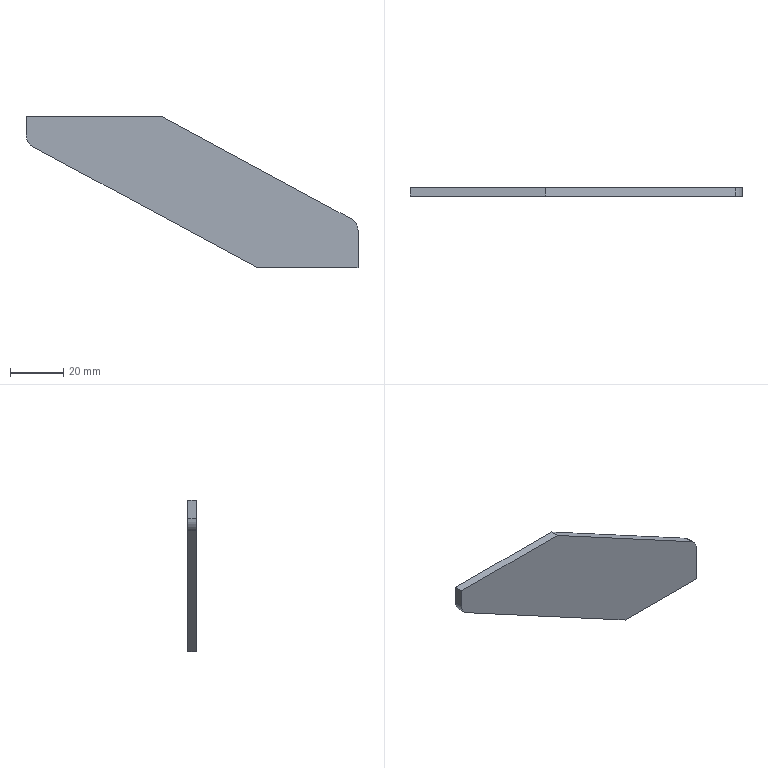Part | SolidWorks | features FlatPattern 1, SMBaseFlange 1, SheetMetal 1 | 1 solid | 10 faces | box 125 x 3.2 x 57 mm | volume 11512 mm3 | plane 8 | cylinder 2 | commonest cylinder face diameters 10 x2
STEP:
#1=CARTESIAN_POINT('',(0.,0.,-7.018));
#2=VERTEX_POINT('',#1);
#3=CARTESIAN_POINT('',(0.,0.,0.));
#4=VERTEX_POINT('',#3);
#5=CARTESIAN_POINT('',(0.,0.,-7.018));
#6=DIRECTION('',(0.,0.,1.));
#7=VECTOR('',#6,1000.);
#8=LINE('',#5,#7);
#9=EDGE_CURVE('',#2,#4,#8,.T.);
#10=ORIENTED_EDGE('',*,*,#9,.F.);
#11=CARTESIAN_POINT('',(0.,-3.2,-7.018));
#12=VERTEX_POINT('',#11);
#13=CARTESIAN_POINT('',(0.,-3.2,-7.018));
#14=DIRECTION('',(0.,1.,0.));
#15=VECTOR('',#14,1000.);
#16=LINE('',#13,#15);
#17=EDGE_CURVE('',#12,#2,#16,.T.);
#18=ORIENTED_EDGE('',*,*,#17,.F.);
#19=CARTESIAN_POINT('',(0.,-3.2,0.));
#20=VERTEX_POINT('',#19);
#21=CARTESIAN_POINT('',(0.,-3.2,-7.018));
#22=DIRECTION('',(0.,0.,1.));
#23=VECTOR('',#22,1000.);
#24=LINE('',#21,#23);
#25=EDGE_CURVE('',#12,#20,#24,.T.);
#26=ORIENTED_EDGE('',*,*,#25,.T.);
#27=CARTESIAN_POINT('',(0.,-3.2,0.));
#28=DIRECTION('',(0.,1.,0.));
#29=VECTOR('',#28,1000.);
#30=LINE('',#27,#29);
#31=EDGE_CURVE('',#20,#4,#30,.T.);
#32=ORIENTED_EDGE('',*,*,#31,.T.);
#33=EDGE_LOOP('',(#10,#18,#26,#32));
#34=FACE_OUTER_BOUND('',#33,.T.);
#35=CARTESIAN_POINT('',(0.,-3.2,-7.018));
#36=DIRECTION('',(-1.,0.,0.));
#37=DIRECTION('',(0.,0.,1.));
#38=AXIS2_PLACEMENT_3D('',#35,#36,#37);
#39=PLANE('',#38);
#40=ADVANCED_FACE('',(#34),#39,.T.);
#41=CARTESIAN_POINT('',(2.623,0.,-11.417));
#42=VERTEX_POINT('',#41);
#43=CARTESIAN_POINT('',(5.,0.,-7.018));
#44=DIRECTION('',(0.,1.,0.));
#45=DIRECTION('',(0.,0.,1.));
#46=AXIS2_PLACEMENT_3D('',#43,#44,#45);
#47=CIRCLE('',#46,5.);
#48=EDGE_CURVE('',#42,#2,#47,.T.);
#49=ORIENTED_EDGE('',*,*,#48,.F.);
#50=CARTESIAN_POINT('',(2.623,-3.2,-11.417));
#51=VERTEX_POINT('',#50);
#52=CARTESIAN_POINT('',(2.623,-3.2,-11.417));
#53=DIRECTION('',(0.,1.,0.));
#54=VECTOR('',#53,1000.);
#55=LINE('',#52,#54);
#56=EDGE_CURVE('',#51,#42,#55,.T.);
#57=ORIENTED_EDGE('',*,*,#56,.F.);
#58=CARTESIAN_POINT('',(5.,-3.2,-7.018));
#59=DIRECTION('',(0.,1.,0.));
#60=DIRECTION('',(0.,0.,1.));
#61=AXIS2_PLACEMENT_3D('',#58,#59,#60);
#62=CIRCLE('',#61,5.);
#63=EDGE_CURVE('',#51,#12,#62,.T.);
#64=ORIENTED_EDGE('',*,*,#63,.T.);
#65=ORIENTED_EDGE('',*,*,#17,.T.);
#66=EDGE_LOOP('',(#49,#57,#64,#65));
#67=FACE_OUTER_BOUND('',#66,.T.);
#68=CARTESIAN_POINT('',(5.,-3.2,-7.018));
#69=DIRECTION('',(0.,1.,0.));
#70=DIRECTION('',(0.,0.,1.));
#71=AXIS2_PLACEMENT_3D('',#68,#69,#70);
#72=CYLINDRICAL_SURFACE('',#71,5.);
#73=ADVANCED_FACE('',(#67),#72,.T.);
#74=CARTESIAN_POINT('',(87.,0.,-57.));
#75=VERTEX_POINT('',#74);
#76=CARTESIAN_POINT('',(87.,0.,-57.));
#77=DIRECTION('',(-0.8798,0.,0.4753));
#78=VECTOR('',#77,1000.);
#79=LINE('',#76,#78);
#80=EDGE_CURVE('',#75,#42,#79,.T.);
#81=ORIENTED_EDGE('',*,*,#80,.F.);
#82=CARTESIAN_POINT('',(87.,-3.2,-57.));
#83=VERTEX_POINT('',#82);
#84=CARTESIAN_POINT('',(87.,-3.2,-57.));
#85=DIRECTION('',(0.,1.,0.));
#86=VECTOR('',#85,1000.);
#87=LINE('',#84,#86);
#88=EDGE_CURVE('',#83,#75,#87,.T.);
#89=ORIENTED_EDGE('',*,*,#88,.F.);
#90=CARTESIAN_POINT('',(87.,-3.2,-57.));
#91=DIRECTION('',(-0.8798,0.,0.4753));
#92=VECTOR('',#91,1000.);
#93=LINE('',#90,#92);
#94=EDGE_CURVE('',#83,#51,#93,.T.);
#95=ORIENTED_EDGE('',*,*,#94,.T.);
#96=ORIENTED_EDGE('',*,*,#56,.T.);
#97=EDGE_LOOP('',(#81,#89,#95,#96));
#98=FACE_OUTER_BOUND('',#97,.T.);
#99=CARTESIAN_POINT('',(87.,-3.2,-57.));
#100=DIRECTION('',(-0.4753,0.,-0.8798));
#101=DIRECTION('',(-0.8798,0.,0.4753));
#102=AXIS2_PLACEMENT_3D('',#99,#100,#101);
#103=PLANE('',#102);
#104=ADVANCED_FACE('',(#98),#103,.T.);
#105=CARTESIAN_POINT('',(125.,0.,-57.));
#106=VERTEX_POINT('',#105);
#107=CARTESIAN_POINT('',(125.,0.,-57.));
#108=DIRECTION('',(-1.,0.,0.));
#109=VECTOR('',#108,1000.);
#110=LINE('',#107,#109);
#111=EDGE_CURVE('',#106,#75,#110,.T.);
#112=ORIENTED_EDGE('',*,*,#111,.F.);
#113=CARTESIAN_POINT('',(125.,-3.2,-57.));
#114=VERTEX_POINT('',#113);
#115=CARTESIAN_POINT('',(125.,-3.2,-57.));
#116=DIRECTION('',(0.,1.,0.));
#117=VECTOR('',#116,1000.);
#118=LINE('',#115,#117);
#119=EDGE_CURVE('',#114,#106,#118,.T.);
#120=ORIENTED_EDGE('',*,*,#119,.F.);
#121=CARTESIAN_POINT('',(125.,-3.2,-57.));
#122=DIRECTION('',(-1.,0.,0.));
#123=VECTOR('',#122,1000.);
#124=LINE('',#121,#123);
#125=EDGE_CURVE('',#114,#83,#124,.T.);
#126=ORIENTED_EDGE('',*,*,#125,.T.);
#127=ORIENTED_EDGE('',*,*,#88,.T.);
#128=EDGE_LOOP('',(#112,#120,#126,#127));
#129=FACE_OUTER_BOUND('',#128,.T.);
#130=CARTESIAN_POINT('',(125.,-3.2,-57.));
#131=DIRECTION('',(0.,0.,-1.));
#132=DIRECTION('',(-1.,0.,0.));
#133=AXIS2_PLACEMENT_3D('',#130,#131,#132);
#134=PLANE('',#133);
#135=ADVANCED_FACE('',(#129),#134,.T.);
#136=CARTESIAN_POINT('',(125.,0.,-42.981));
#137=VERTEX_POINT('',#136);
#138=CARTESIAN_POINT('',(125.,0.,-42.981));
#139=DIRECTION('',(0.,0.,-1.));
#140=VECTOR('',#139,1000.);
#141=LINE('',#138,#140);
#142=EDGE_CURVE('',#137,#106,#141,.T.);
#143=ORIENTED_EDGE('',*,*,#142,.F.);
#144=CARTESIAN_POINT('',(125.,-3.2,-42.981));
#145=VERTEX_POINT('',#144);
#146=CARTESIAN_POINT('',(125.,-3.2,-42.981));
#147=DIRECTION('',(0.,1.,0.));
#148=VECTOR('',#147,1000.);
#149=LINE('',#146,#148);
#150=EDGE_CURVE('',#145,#137,#149,.T.);
#151=ORIENTED_EDGE('',*,*,#150,.F.);
#152=CARTESIAN_POINT('',(125.,-3.2,-42.981));
#153=DIRECTION('',(0.,0.,-1.));
#154=VECTOR('',#153,1000.);
#155=LINE('',#152,#154);
#156=EDGE_CURVE('',#145,#114,#155,.T.);
#157=ORIENTED_EDGE('',*,*,#156,.T.);
#158=ORIENTED_EDGE('',*,*,#119,.T.);
#159=EDGE_LOOP('',(#143,#151,#157,#158));
#160=FACE_OUTER_BOUND('',#159,.T.);
#161=CARTESIAN_POINT('',(125.,-3.2,-42.981));
#162=DIRECTION('',(1.,0.,0.));
#163=DIRECTION('',(0.,0.,-1.));
#164=AXIS2_PLACEMENT_3D('',#161,#162,#163);
#165=PLANE('',#164);
#166=ADVANCED_FACE('',(#160),#165,.T.);
#167=CARTESIAN_POINT('',(122.378,0.,-38.582));
#168=VERTEX_POINT('',#167);
#169=CARTESIAN_POINT('',(120.,0.,-42.981));
#170=DIRECTION('',(0.,1.,0.));
#171=DIRECTION('',(0.,0.,1.));
#172=AXIS2_PLACEMENT_3D('',#169,#170,#171);
#173=CIRCLE('',#172,5.);
#174=EDGE_CURVE('',#168,#137,#173,.T.);
#175=ORIENTED_EDGE('',*,*,#174,.F.);
#176=CARTESIAN_POINT('',(122.378,-3.2,-38.582));
#177=VERTEX_POINT('',#176);
#178=CARTESIAN_POINT('',(122.378,-3.2,-38.582));
#179=DIRECTION('',(0.,1.,0.));
#180=VECTOR('',#179,1000.);
#181=LINE('',#178,#180);
#182=EDGE_CURVE('',#177,#168,#181,.T.);
#183=ORIENTED_EDGE('',*,*,#182,.F.);
#184=CARTESIAN_POINT('',(120.,-3.2,-42.981));
#185=DIRECTION('',(0.,1.,0.));
#186=DIRECTION('',(0.,0.,1.));
#187=AXIS2_PLACEMENT_3D('',#184,#185,#186);
#188=CIRCLE('',#187,5.);
#189=EDGE_CURVE('',#177,#145,#188,.T.);
#190=ORIENTED_EDGE('',*,*,#189,.T.);
#191=ORIENTED_EDGE('',*,*,#150,.T.);
#192=EDGE_LOOP('',(#175,#183,#190,#191));
#193=FACE_OUTER_BOUND('',#192,.T.);
#194=CARTESIAN_POINT('',(120.,-3.2,-42.981));
#195=DIRECTION('',(0.,1.,0.));
#196=DIRECTION('',(0.,0.,1.));
#197=AXIS2_PLACEMENT_3D('',#194,#195,#196);
#198=CYLINDRICAL_SURFACE('',#197,5.);
#199=ADVANCED_FACE('',(#193),#198,.T.);
#200=CARTESIAN_POINT('',(51.,0.,0.));
#201=VERTEX_POINT('',#200);
#202=CARTESIAN_POINT('',(51.,0.,0.));
#203=DIRECTION('',(0.8797,0.,-0.4755));
#204=VECTOR('',#203,1000.);
#205=LINE('',#202,#204);
#206=EDGE_CURVE('',#201,#168,#205,.T.);
#207=ORIENTED_EDGE('',*,*,#206,.F.);
#208=CARTESIAN_POINT('',(51.,-3.2,0.));
#209=VERTEX_POINT('',#208);
#210=CARTESIAN_POINT('',(51.,-3.2,0.));
#211=DIRECTION('',(0.,1.,0.));
#212=VECTOR('',#211,1000.);
#213=LINE('',#210,#212);
#214=EDGE_CURVE('',#209,#201,#213,.T.);
#215=ORIENTED_EDGE('',*,*,#214,.F.);
#216=CARTESIAN_POINT('',(51.,-3.2,0.));
#217=DIRECTION('',(0.8797,0.,-0.4755));
#218=VECTOR('',#217,1000.);
#219=LINE('',#216,#218);
#220=EDGE_CURVE('',#209,#177,#219,.T.);
#221=ORIENTED_EDGE('',*,*,#220,.T.);
#222=ORIENTED_EDGE('',*,*,#182,.T.);
#223=EDGE_LOOP('',(#207,#215,#221,#222));
#224=FACE_OUTER_BOUND('',#223,.T.);
#225=CARTESIAN_POINT('',(51.,-3.2,0.));
#226=DIRECTION('',(0.4755,0.,0.8797));
#227=DIRECTION('',(0.8797,0.,-0.4755));
#228=AXIS2_PLACEMENT_3D('',#225,#226,#227);
#229=PLANE('',#228);
#230=ADVANCED_FACE('',(#224),#229,.T.);
#231=CARTESIAN_POINT('',(0.,0.,0.));
#232=DIRECTION('',(1.,0.,0.));
#233=VECTOR('',#232,1000.);
#234=LINE('',#231,#233);
#235=EDGE_CURVE('',#4,#201,#234,.T.);
#236=ORIENTED_EDGE('',*,*,#235,.F.);
#237=ORIENTED_EDGE('',*,*,#31,.F.);
#238=CARTESIAN_POINT('',(0.,-3.2,0.));
#239=DIRECTION('',(1.,0.,0.));
#240=VECTOR('',#239,1000.);
#241=LINE('',#238,#240);
#242=EDGE_CURVE('',#20,#209,#241,.T.);
#243=ORIENTED_EDGE('',*,*,#242,.T.);
#244=ORIENTED_EDGE('',*,*,#214,.T.);
#245=EDGE_LOOP('',(#236,#237,#243,#244));
#246=FACE_OUTER_BOUND('',#245,.T.);
#247=CARTESIAN_POINT('',(0.,-3.2,0.));
#248=DIRECTION('',(0.,0.,1.));
#249=DIRECTION('',(1.,0.,0.));
#250=AXIS2_PLACEMENT_3D('',#247,#248,#249);
#251=PLANE('',#250);
#252=ADVANCED_FACE('',(#246),#251,.T.);
#253=ORIENTED_EDGE('',*,*,#25,.F.);
#254=ORIENTED_EDGE('',*,*,#63,.F.);
#255=ORIENTED_EDGE('',*,*,#94,.F.);
#256=ORIENTED_EDGE('',*,*,#125,.F.);
#257=ORIENTED_EDGE('',*,*,#156,.F.);
#258=ORIENTED_EDGE('',*,*,#189,.F.);
#259=ORIENTED_EDGE('',*,*,#220,.F.);
#260=ORIENTED_EDGE('',*,*,#242,.F.);
#261=EDGE_LOOP('',(#253,#254,#255,#256,#257,#258,#259,#260));
#262=FACE_OUTER_BOUND('',#261,.T.);
#263=CARTESIAN_POINT('',(120.,-3.2,-42.981));
#264=DIRECTION('',(0.,1.,0.));
#265=DIRECTION('',(0.,0.,1.));
#266=AXIS2_PLACEMENT_3D('',#263,#264,#265);
#267=PLANE('',#266);
#268=ADVANCED_FACE('',(#262),#267,.F.);
#269=ORIENTED_EDGE('',*,*,#9,.T.);
#270=ORIENTED_EDGE('',*,*,#235,.T.);
#271=ORIENTED_EDGE('',*,*,#206,.T.);
#272=ORIENTED_EDGE('',*,*,#174,.T.);
#273=ORIENTED_EDGE('',*,*,#142,.T.);
#274=ORIENTED_EDGE('',*,*,#111,.T.);
#275=ORIENTED_EDGE('',*,*,#80,.T.);
#276=ORIENTED_EDGE('',*,*,#48,.T.);
#277=EDGE_LOOP('',(#269,#270,#271,#272,#273,#274,#275,#276));
#278=FACE_OUTER_BOUND('',#277,.T.);
#279=CARTESIAN_POINT('',(120.,0.,-42.981));
#280=DIRECTION('',(0.,1.,0.));
#281=DIRECTION('',(0.,0.,1.));
#282=AXIS2_PLACEMENT_3D('',#279,#280,#281);
#283=PLANE('',#282);
#284=ADVANCED_FACE('',(#278),#283,.T.);
#285=CLOSED_SHELL('',(#40,#73,#104,#135,#166,#199,#230,#252,#268,#284));
#286=MANIFOLD_SOLID_BREP('',#285);
#287=CARTESIAN_POINT('',(0.,0.,0.));
#288=DIRECTION('',(0.,0.,1.));
#289=DIRECTION('',(1.,0.,0.));
#290=AXIS2_PLACEMENT_3D('',#287,#288,#289);
#291=(LENGTH_UNIT()NAMED_UNIT(*)SI_UNIT(.MILLI.,.METRE.));
#292=UNCERTAINTY_MEASURE_WITH_UNIT(LENGTH_MEASURE(0.00001),#291,'','');
#293=(NAMED_UNIT(*)PLANE_ANGLE_UNIT()SI_UNIT($,.RADIAN.));
#294=(NAMED_UNIT(*)SI_UNIT($,.STERADIAN.)SOLID_ANGLE_UNIT());
#295=(GEOMETRIC_REPRESENTATION_CONTEXT(3)GLOBAL_UNCERTAINTY_ASSIGNED_CONTEXT((#292))GLOBAL_UNIT_ASSIGNED_CONTEXT((#291,#293,#294))REPRESENTATION_CONTEXT('',''));
#296=ADVANCED_BREP_SHAPE_REPRESENTATION('',(#286,#290),#295);